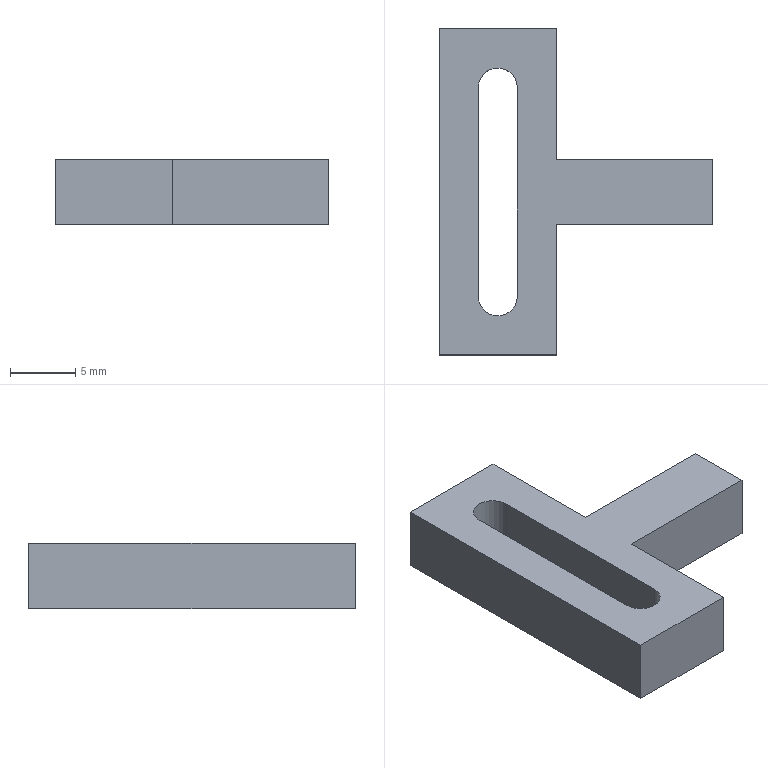Part | SolidWorks | features Extrusion 1 | 1 solid | 14 faces | box 21 x 25 x 5 mm | volume 1150 mm3 | plane 12 | cylinder 2 | commonest cylinder face diameters 3 x2
STEP:
#1=CARTESIAN_POINT('',(0.,-2.5,2.5));
#2=VERTEX_POINT('',#1);
#3=CARTESIAN_POINT('',(0.,2.5,2.5));
#4=VERTEX_POINT('',#3);
#5=CARTESIAN_POINT('',(0.,-2.5,2.5));
#6=DIRECTION('',(0.,1.,0.));
#7=VECTOR('',#6,1000.);
#8=LINE('',#5,#7);
#9=EDGE_CURVE('',#2,#4,#8,.T.);
#10=ORIENTED_EDGE('',*,*,#9,.T.);
#11=CARTESIAN_POINT('',(-12.,2.5,2.5));
#12=VERTEX_POINT('',#11);
#13=CARTESIAN_POINT('',(0.,2.5,2.5));
#14=DIRECTION('',(-1.,0.,0.));
#15=VECTOR('',#14,1000.);
#16=LINE('',#13,#15);
#17=EDGE_CURVE('',#4,#12,#16,.T.);
#18=ORIENTED_EDGE('',*,*,#17,.T.);
#19=CARTESIAN_POINT('',(-12.,12.5,2.5));
#20=VERTEX_POINT('',#19);
#21=CARTESIAN_POINT('',(-12.,2.5,2.5));
#22=DIRECTION('',(0.,1.,0.));
#23=VECTOR('',#22,1000.);
#24=LINE('',#21,#23);
#25=EDGE_CURVE('',#12,#20,#24,.T.);
#26=ORIENTED_EDGE('',*,*,#25,.T.);
#27=CARTESIAN_POINT('',(-21.,12.5,2.5));
#28=VERTEX_POINT('',#27);
#29=CARTESIAN_POINT('',(-12.,12.5,2.5));
#30=DIRECTION('',(-1.,0.,0.));
#31=VECTOR('',#30,1000.);
#32=LINE('',#29,#31);
#33=EDGE_CURVE('',#20,#28,#32,.T.);
#34=ORIENTED_EDGE('',*,*,#33,.T.);
#35=CARTESIAN_POINT('',(-21.,-12.5,2.5));
#36=VERTEX_POINT('',#35);
#37=CARTESIAN_POINT('',(-21.,12.5,2.5));
#38=DIRECTION('',(0.,-1.,0.));
#39=VECTOR('',#38,1000.);
#40=LINE('',#37,#39);
#41=EDGE_CURVE('',#28,#36,#40,.T.);
#42=ORIENTED_EDGE('',*,*,#41,.T.);
#43=CARTESIAN_POINT('',(-12.,-12.5,2.5));
#44=VERTEX_POINT('',#43);
#45=CARTESIAN_POINT('',(-21.,-12.5,2.5));
#46=DIRECTION('',(1.,0.,0.));
#47=VECTOR('',#46,1000.);
#48=LINE('',#45,#47);
#49=EDGE_CURVE('',#36,#44,#48,.T.);
#50=ORIENTED_EDGE('',*,*,#49,.T.);
#51=CARTESIAN_POINT('',(-12.,-2.5,2.5));
#52=VERTEX_POINT('',#51);
#53=CARTESIAN_POINT('',(-12.,-12.5,2.5));
#54=DIRECTION('',(0.,1.,0.));
#55=VECTOR('',#54,1000.);
#56=LINE('',#53,#55);
#57=EDGE_CURVE('',#44,#52,#56,.T.);
#58=ORIENTED_EDGE('',*,*,#57,.T.);
#59=CARTESIAN_POINT('',(-12.,-2.5,2.5));
#60=DIRECTION('',(1.,0.,0.));
#61=VECTOR('',#60,1000.);
#62=LINE('',#59,#61);
#63=EDGE_CURVE('',#52,#2,#62,.T.);
#64=ORIENTED_EDGE('',*,*,#63,.T.);
#65=EDGE_LOOP('',(#10,#18,#26,#34,#42,#50,#58,#64));
#66=FACE_OUTER_BOUND('',#65,.T.);
#67=CARTESIAN_POINT('',(-15.,-8.,2.5));
#68=VERTEX_POINT('',#67);
#69=CARTESIAN_POINT('',(-15.,8.,2.5));
#70=VERTEX_POINT('',#69);
#71=CARTESIAN_POINT('',(-15.,-8.,2.5));
#72=DIRECTION('',(0.,1.,0.));
#73=VECTOR('',#72,1000.);
#74=LINE('',#71,#73);
#75=EDGE_CURVE('',#68,#70,#74,.T.);
#76=ORIENTED_EDGE('',*,*,#75,.F.);
#77=CARTESIAN_POINT('',(-18.,-8.,2.5));
#78=VERTEX_POINT('',#77);
#79=CARTESIAN_POINT('',(-16.5,-8.,2.5));
#80=DIRECTION('',(0.,0.,1.));
#81=DIRECTION('',(1.,0.,0.));
#82=AXIS2_PLACEMENT_3D('',#79,#80,#81);
#83=CIRCLE('',#82,1.5);
#84=EDGE_CURVE('',#78,#68,#83,.T.);
#85=ORIENTED_EDGE('',*,*,#84,.F.);
#86=CARTESIAN_POINT('',(-18.,8.,2.5));
#87=VERTEX_POINT('',#86);
#88=CARTESIAN_POINT('',(-18.,-8.,2.5));
#89=DIRECTION('',(0.,-1.,0.));
#90=VECTOR('',#89,1000.);
#91=LINE('',#88,#90);
#92=EDGE_CURVE('',#87,#78,#91,.T.);
#93=ORIENTED_EDGE('',*,*,#92,.F.);
#94=CARTESIAN_POINT('',(-16.5,8.,2.5));
#95=DIRECTION('',(0.,0.,1.));
#96=DIRECTION('',(1.,0.,0.));
#97=AXIS2_PLACEMENT_3D('',#94,#95,#96);
#98=CIRCLE('',#97,1.5);
#99=EDGE_CURVE('',#70,#87,#98,.T.);
#100=ORIENTED_EDGE('',*,*,#99,.F.);
#101=EDGE_LOOP('',(#76,#85,#93,#100));
#102=FACE_BOUND('',#101,.T.);
#103=CARTESIAN_POINT('',(0.,0.,2.5));
#104=DIRECTION('',(0.,0.,1.));
#105=DIRECTION('',(1.,0.,0.));
#106=AXIS2_PLACEMENT_3D('',#103,#104,#105);
#107=PLANE('',#106);
#108=ADVANCED_FACE('',(#66,#102),#107,.T.);
#109=CARTESIAN_POINT('',(0.,-2.5,-2.5));
#110=VERTEX_POINT('',#109);
#111=CARTESIAN_POINT('',(0.,2.5,-2.5));
#112=VERTEX_POINT('',#111);
#113=CARTESIAN_POINT('',(0.,0.,-2.5));
#114=DIRECTION('',(0.,1.,0.));
#115=VECTOR('',#114,1000.);
#116=LINE('',#113,#115);
#117=EDGE_CURVE('',#110,#112,#116,.T.);
#118=ORIENTED_EDGE('',*,*,#117,.F.);
#119=CARTESIAN_POINT('',(-12.,-2.5,-2.5));
#120=VERTEX_POINT('',#119);
#121=CARTESIAN_POINT('',(-12.,-2.5,-2.5));
#122=DIRECTION('',(1.,0.,0.));
#123=VECTOR('',#122,1000.);
#124=LINE('',#121,#123);
#125=EDGE_CURVE('',#120,#110,#124,.T.);
#126=ORIENTED_EDGE('',*,*,#125,.F.);
#127=CARTESIAN_POINT('',(-12.,-12.5,-2.5));
#128=VERTEX_POINT('',#127);
#129=CARTESIAN_POINT('',(-12.,-12.5,-2.5));
#130=DIRECTION('',(0.,1.,0.));
#131=VECTOR('',#130,1000.);
#132=LINE('',#129,#131);
#133=EDGE_CURVE('',#128,#120,#132,.T.);
#134=ORIENTED_EDGE('',*,*,#133,.F.);
#135=CARTESIAN_POINT('',(-21.,-12.5,-2.5));
#136=VERTEX_POINT('',#135);
#137=CARTESIAN_POINT('',(-21.,-12.5,-2.5));
#138=DIRECTION('',(1.,0.,0.));
#139=VECTOR('',#138,1000.);
#140=LINE('',#137,#139);
#141=EDGE_CURVE('',#136,#128,#140,.T.);
#142=ORIENTED_EDGE('',*,*,#141,.F.);
#143=CARTESIAN_POINT('',(-21.,12.5,-2.5));
#144=VERTEX_POINT('',#143);
#145=CARTESIAN_POINT('',(-21.,12.5,-2.5));
#146=DIRECTION('',(0.,-1.,0.));
#147=VECTOR('',#146,1000.);
#148=LINE('',#145,#147);
#149=EDGE_CURVE('',#144,#136,#148,.T.);
#150=ORIENTED_EDGE('',*,*,#149,.F.);
#151=CARTESIAN_POINT('',(-12.,12.5,-2.5));
#152=VERTEX_POINT('',#151);
#153=CARTESIAN_POINT('',(-12.,12.5,-2.5));
#154=DIRECTION('',(-1.,0.,0.));
#155=VECTOR('',#154,1000.);
#156=LINE('',#153,#155);
#157=EDGE_CURVE('',#152,#144,#156,.T.);
#158=ORIENTED_EDGE('',*,*,#157,.F.);
#159=CARTESIAN_POINT('',(-12.,2.5,-2.5));
#160=VERTEX_POINT('',#159);
#161=CARTESIAN_POINT('',(-12.,2.5,-2.5));
#162=DIRECTION('',(0.,1.,0.));
#163=VECTOR('',#162,1000.);
#164=LINE('',#161,#163);
#165=EDGE_CURVE('',#160,#152,#164,.T.);
#166=ORIENTED_EDGE('',*,*,#165,.F.);
#167=CARTESIAN_POINT('',(0.,2.5,-2.5));
#168=DIRECTION('',(-1.,0.,0.));
#169=VECTOR('',#168,1000.);
#170=LINE('',#167,#169);
#171=EDGE_CURVE('',#112,#160,#170,.T.);
#172=ORIENTED_EDGE('',*,*,#171,.F.);
#173=EDGE_LOOP('',(#118,#126,#134,#142,#150,#158,#166,#172));
#174=FACE_OUTER_BOUND('',#173,.T.);
#175=CARTESIAN_POINT('',(-18.,-8.,-2.5));
#176=VERTEX_POINT('',#175);
#177=CARTESIAN_POINT('',(-15.,-8.,-2.5));
#178=VERTEX_POINT('',#177);
#179=CARTESIAN_POINT('',(-16.5,-8.,-2.5));
#180=DIRECTION('',(0.,0.,1.));
#181=DIRECTION('',(1.,0.,0.));
#182=AXIS2_PLACEMENT_3D('',#179,#180,#181);
#183=CIRCLE('',#182,1.5);
#184=EDGE_CURVE('',#176,#178,#183,.T.);
#185=ORIENTED_EDGE('',*,*,#184,.T.);
#186=CARTESIAN_POINT('',(-15.,8.,-2.5));
#187=VERTEX_POINT('',#186);
#188=CARTESIAN_POINT('',(-15.,-8.,-2.5));
#189=DIRECTION('',(0.,1.,0.));
#190=VECTOR('',#189,1000.);
#191=LINE('',#188,#190);
#192=EDGE_CURVE('',#178,#187,#191,.T.);
#193=ORIENTED_EDGE('',*,*,#192,.T.);
#194=CARTESIAN_POINT('',(-18.,8.,-2.5));
#195=VERTEX_POINT('',#194);
#196=CARTESIAN_POINT('',(-16.5,8.,-2.5));
#197=DIRECTION('',(0.,0.,1.));
#198=DIRECTION('',(1.,0.,0.));
#199=AXIS2_PLACEMENT_3D('',#196,#197,#198);
#200=CIRCLE('',#199,1.5);
#201=EDGE_CURVE('',#187,#195,#200,.T.);
#202=ORIENTED_EDGE('',*,*,#201,.T.);
#203=CARTESIAN_POINT('',(-18.,-8.,-2.5));
#204=DIRECTION('',(0.,-1.,0.));
#205=VECTOR('',#204,1000.);
#206=LINE('',#203,#205);
#207=EDGE_CURVE('',#195,#176,#206,.T.);
#208=ORIENTED_EDGE('',*,*,#207,.T.);
#209=EDGE_LOOP('',(#185,#193,#202,#208));
#210=FACE_BOUND('',#209,.T.);
#211=CARTESIAN_POINT('',(0.,0.,-2.5));
#212=DIRECTION('',(0.,0.,1.));
#213=DIRECTION('',(1.,0.,0.));
#214=AXIS2_PLACEMENT_3D('',#211,#212,#213);
#215=PLANE('',#214);
#216=ADVANCED_FACE('',(#174,#210),#215,.F.);
#217=ORIENTED_EDGE('',*,*,#117,.T.);
#218=CARTESIAN_POINT('',(0.,2.5,2.5));
#219=DIRECTION('',(0.,0.,-1.));
#220=VECTOR('',#219,1000.);
#221=LINE('',#218,#220);
#222=EDGE_CURVE('',#4,#112,#221,.T.);
#223=ORIENTED_EDGE('',*,*,#222,.F.);
#224=ORIENTED_EDGE('',*,*,#9,.F.);
#225=CARTESIAN_POINT('',(0.,-2.5,2.5));
#226=DIRECTION('',(0.,0.,-1.));
#227=VECTOR('',#226,1000.);
#228=LINE('',#225,#227);
#229=EDGE_CURVE('',#2,#110,#228,.T.);
#230=ORIENTED_EDGE('',*,*,#229,.T.);
#231=EDGE_LOOP('',(#217,#223,#224,#230));
#232=FACE_OUTER_BOUND('',#231,.T.);
#233=CARTESIAN_POINT('',(0.,0.,2.5));
#234=DIRECTION('',(-1.,0.,0.));
#235=DIRECTION('',(0.,0.,1.));
#236=AXIS2_PLACEMENT_3D('',#233,#234,#235);
#237=PLANE('',#236);
#238=ADVANCED_FACE('',(#232),#237,.F.);
#239=ORIENTED_EDGE('',*,*,#171,.T.);
#240=CARTESIAN_POINT('',(-12.,2.5,2.5));
#241=DIRECTION('',(0.,0.,-1.));
#242=VECTOR('',#241,1000.);
#243=LINE('',#240,#242);
#244=EDGE_CURVE('',#12,#160,#243,.T.);
#245=ORIENTED_EDGE('',*,*,#244,.F.);
#246=ORIENTED_EDGE('',*,*,#17,.F.);
#247=ORIENTED_EDGE('',*,*,#222,.T.);
#248=EDGE_LOOP('',(#239,#245,#246,#247));
#249=FACE_OUTER_BOUND('',#248,.T.);
#250=CARTESIAN_POINT('',(0.,2.5,2.5));
#251=DIRECTION('',(0.,-1.,0.));
#252=DIRECTION('',(1.,0.,0.));
#253=AXIS2_PLACEMENT_3D('',#250,#251,#252);
#254=PLANE('',#253);
#255=ADVANCED_FACE('',(#249),#254,.F.);
#256=ORIENTED_EDGE('',*,*,#165,.T.);
#257=CARTESIAN_POINT('',(-12.,12.5,2.5));
#258=DIRECTION('',(0.,0.,-1.));
#259=VECTOR('',#258,1000.);
#260=LINE('',#257,#259);
#261=EDGE_CURVE('',#20,#152,#260,.T.);
#262=ORIENTED_EDGE('',*,*,#261,.F.);
#263=ORIENTED_EDGE('',*,*,#25,.F.);
#264=ORIENTED_EDGE('',*,*,#244,.T.);
#265=EDGE_LOOP('',(#256,#262,#263,#264));
#266=FACE_OUTER_BOUND('',#265,.T.);
#267=CARTESIAN_POINT('',(-12.,2.5,2.5));
#268=DIRECTION('',(-1.,0.,0.));
#269=DIRECTION('',(0.,0.,1.));
#270=AXIS2_PLACEMENT_3D('',#267,#268,#269);
#271=PLANE('',#270);
#272=ADVANCED_FACE('',(#266),#271,.F.);
#273=ORIENTED_EDGE('',*,*,#157,.T.);
#274=CARTESIAN_POINT('',(-21.,12.5,2.5));
#275=DIRECTION('',(0.,0.,-1.));
#276=VECTOR('',#275,1000.);
#277=LINE('',#274,#276);
#278=EDGE_CURVE('',#28,#144,#277,.T.);
#279=ORIENTED_EDGE('',*,*,#278,.F.);
#280=ORIENTED_EDGE('',*,*,#33,.F.);
#281=ORIENTED_EDGE('',*,*,#261,.T.);
#282=EDGE_LOOP('',(#273,#279,#280,#281));
#283=FACE_OUTER_BOUND('',#282,.T.);
#284=CARTESIAN_POINT('',(-12.,12.5,2.5));
#285=DIRECTION('',(0.,-1.,0.));
#286=DIRECTION('',(1.,0.,0.));
#287=AXIS2_PLACEMENT_3D('',#284,#285,#286);
#288=PLANE('',#287);
#289=ADVANCED_FACE('',(#283),#288,.F.);
#290=ORIENTED_EDGE('',*,*,#149,.T.);
#291=CARTESIAN_POINT('',(-21.,-12.5,2.5));
#292=DIRECTION('',(0.,0.,-1.));
#293=VECTOR('',#292,1000.);
#294=LINE('',#291,#293);
#295=EDGE_CURVE('',#36,#136,#294,.T.);
#296=ORIENTED_EDGE('',*,*,#295,.F.);
#297=ORIENTED_EDGE('',*,*,#41,.F.);
#298=ORIENTED_EDGE('',*,*,#278,.T.);
#299=EDGE_LOOP('',(#290,#296,#297,#298));
#300=FACE_OUTER_BOUND('',#299,.T.);
#301=CARTESIAN_POINT('',(-21.,12.5,2.5));
#302=DIRECTION('',(1.,0.,0.));
#303=DIRECTION('',(0.,1.,0.));
#304=AXIS2_PLACEMENT_3D('',#301,#302,#303);
#305=PLANE('',#304);
#306=ADVANCED_FACE('',(#300),#305,.F.);
#307=ORIENTED_EDGE('',*,*,#141,.T.);
#308=CARTESIAN_POINT('',(-12.,-12.5,2.5));
#309=DIRECTION('',(0.,0.,-1.));
#310=VECTOR('',#309,1000.);
#311=LINE('',#308,#310);
#312=EDGE_CURVE('',#44,#128,#311,.T.);
#313=ORIENTED_EDGE('',*,*,#312,.F.);
#314=ORIENTED_EDGE('',*,*,#49,.F.);
#315=ORIENTED_EDGE('',*,*,#295,.T.);
#316=EDGE_LOOP('',(#307,#313,#314,#315));
#317=FACE_OUTER_BOUND('',#316,.T.);
#318=CARTESIAN_POINT('',(-21.,-12.5,2.5));
#319=DIRECTION('',(0.,1.,0.));
#320=DIRECTION('',(0.,0.,1.));
#321=AXIS2_PLACEMENT_3D('',#318,#319,#320);
#322=PLANE('',#321);
#323=ADVANCED_FACE('',(#317),#322,.F.);
#324=ORIENTED_EDGE('',*,*,#133,.T.);
#325=CARTESIAN_POINT('',(-12.,-2.5,2.5));
#326=DIRECTION('',(0.,0.,-1.));
#327=VECTOR('',#326,1000.);
#328=LINE('',#325,#327);
#329=EDGE_CURVE('',#52,#120,#328,.T.);
#330=ORIENTED_EDGE('',*,*,#329,.F.);
#331=ORIENTED_EDGE('',*,*,#57,.F.);
#332=ORIENTED_EDGE('',*,*,#312,.T.);
#333=EDGE_LOOP('',(#324,#330,#331,#332));
#334=FACE_OUTER_BOUND('',#333,.T.);
#335=CARTESIAN_POINT('',(-12.,-12.5,2.5));
#336=DIRECTION('',(-1.,0.,0.));
#337=DIRECTION('',(0.,0.,1.));
#338=AXIS2_PLACEMENT_3D('',#335,#336,#337);
#339=PLANE('',#338);
#340=ADVANCED_FACE('',(#334),#339,.F.);
#341=ORIENTED_EDGE('',*,*,#125,.T.);
#342=ORIENTED_EDGE('',*,*,#229,.F.);
#343=ORIENTED_EDGE('',*,*,#63,.F.);
#344=ORIENTED_EDGE('',*,*,#329,.T.);
#345=EDGE_LOOP('',(#341,#342,#343,#344));
#346=FACE_OUTER_BOUND('',#345,.T.);
#347=CARTESIAN_POINT('',(-12.,-2.5,2.5));
#348=DIRECTION('',(0.,1.,0.));
#349=DIRECTION('',(0.,0.,1.));
#350=AXIS2_PLACEMENT_3D('',#347,#348,#349);
#351=PLANE('',#350);
#352=ADVANCED_FACE('',(#346),#351,.F.);
#353=ORIENTED_EDGE('',*,*,#184,.F.);
#354=CARTESIAN_POINT('',(-18.,-8.,2.5));
#355=DIRECTION('',(0.,0.,-1.));
#356=VECTOR('',#355,1000.);
#357=LINE('',#354,#356);
#358=EDGE_CURVE('',#78,#176,#357,.T.);
#359=ORIENTED_EDGE('',*,*,#358,.F.);
#360=ORIENTED_EDGE('',*,*,#84,.T.);
#361=CARTESIAN_POINT('',(-15.,-8.,2.5));
#362=DIRECTION('',(0.,0.,-1.));
#363=VECTOR('',#362,1000.);
#364=LINE('',#361,#363);
#365=EDGE_CURVE('',#68,#178,#364,.T.);
#366=ORIENTED_EDGE('',*,*,#365,.T.);
#367=EDGE_LOOP('',(#353,#359,#360,#366));
#368=FACE_OUTER_BOUND('',#367,.T.);
#369=CARTESIAN_POINT('',(-16.5,-8.,2.5));
#370=DIRECTION('',(0.,0.,-1.));
#371=DIRECTION('',(-1.,0.,0.));
#372=AXIS2_PLACEMENT_3D('',#369,#370,#371);
#373=CYLINDRICAL_SURFACE('',#372,1.5);
#374=ADVANCED_FACE('',(#368),#373,.F.);
#375=ORIENTED_EDGE('',*,*,#192,.F.);
#376=ORIENTED_EDGE('',*,*,#365,.F.);
#377=ORIENTED_EDGE('',*,*,#75,.T.);
#378=CARTESIAN_POINT('',(-15.,8.,2.5));
#379=DIRECTION('',(0.,0.,-1.));
#380=VECTOR('',#379,1000.);
#381=LINE('',#378,#380);
#382=EDGE_CURVE('',#70,#187,#381,.T.);
#383=ORIENTED_EDGE('',*,*,#382,.T.);
#384=EDGE_LOOP('',(#375,#376,#377,#383));
#385=FACE_OUTER_BOUND('',#384,.T.);
#386=CARTESIAN_POINT('',(-15.,-8.,2.5));
#387=DIRECTION('',(-1.,0.,0.));
#388=DIRECTION('',(0.,0.,1.));
#389=AXIS2_PLACEMENT_3D('',#386,#387,#388);
#390=PLANE('',#389);
#391=ADVANCED_FACE('',(#385),#390,.T.);
#392=ORIENTED_EDGE('',*,*,#201,.F.);
#393=ORIENTED_EDGE('',*,*,#382,.F.);
#394=ORIENTED_EDGE('',*,*,#99,.T.);
#395=CARTESIAN_POINT('',(-18.,8.,2.5));
#396=DIRECTION('',(0.,0.,-1.));
#397=VECTOR('',#396,1000.);
#398=LINE('',#395,#397);
#399=EDGE_CURVE('',#87,#195,#398,.T.);
#400=ORIENTED_EDGE('',*,*,#399,.T.);
#401=EDGE_LOOP('',(#392,#393,#394,#400));
#402=FACE_OUTER_BOUND('',#401,.T.);
#403=CARTESIAN_POINT('',(-16.5,8.,2.5));
#404=DIRECTION('',(0.,0.,-1.));
#405=DIRECTION('',(-1.,0.,0.));
#406=AXIS2_PLACEMENT_3D('',#403,#404,#405);
#407=CYLINDRICAL_SURFACE('',#406,1.5);
#408=ADVANCED_FACE('',(#402),#407,.F.);
#409=ORIENTED_EDGE('',*,*,#207,.F.);
#410=ORIENTED_EDGE('',*,*,#399,.F.);
#411=ORIENTED_EDGE('',*,*,#92,.T.);
#412=ORIENTED_EDGE('',*,*,#358,.T.);
#413=EDGE_LOOP('',(#409,#410,#411,#412));
#414=FACE_OUTER_BOUND('',#413,.T.);
#415=CARTESIAN_POINT('',(-18.,-8.,2.5));
#416=DIRECTION('',(1.,0.,0.));
#417=DIRECTION('',(0.,0.,-1.));
#418=AXIS2_PLACEMENT_3D('',#415,#416,#417);
#419=PLANE('',#418);
#420=ADVANCED_FACE('',(#414),#419,.T.);
#421=CLOSED_SHELL('',(#108,#216,#238,#255,#272,#289,#306,#323,#340,#352,#374,#391,#408,#420));
#422=MANIFOLD_SOLID_BREP('',#421);
#423=CARTESIAN_POINT('',(0.,0.,0.));
#424=DIRECTION('',(0.,0.,1.));
#425=DIRECTION('',(1.,0.,0.));
#426=AXIS2_PLACEMENT_3D('',#423,#424,#425);
#427=(LENGTH_UNIT()NAMED_UNIT(*)SI_UNIT(.MILLI.,.METRE.));
#428=UNCERTAINTY_MEASURE_WITH_UNIT(LENGTH_MEASURE(0.00001),#427,'','');
#429=(NAMED_UNIT(*)PLANE_ANGLE_UNIT()SI_UNIT($,.RADIAN.));
#430=(NAMED_UNIT(*)SI_UNIT($,.STERADIAN.)SOLID_ANGLE_UNIT());
#431=(GEOMETRIC_REPRESENTATION_CONTEXT(3)GLOBAL_UNCERTAINTY_ASSIGNED_CONTEXT((#428))GLOBAL_UNIT_ASSIGNED_CONTEXT((#427,#429,#430))REPRESENTATION_CONTEXT('',''));
#432=ADVANCED_BREP_SHAPE_REPRESENTATION('',(#422,#426),#431);